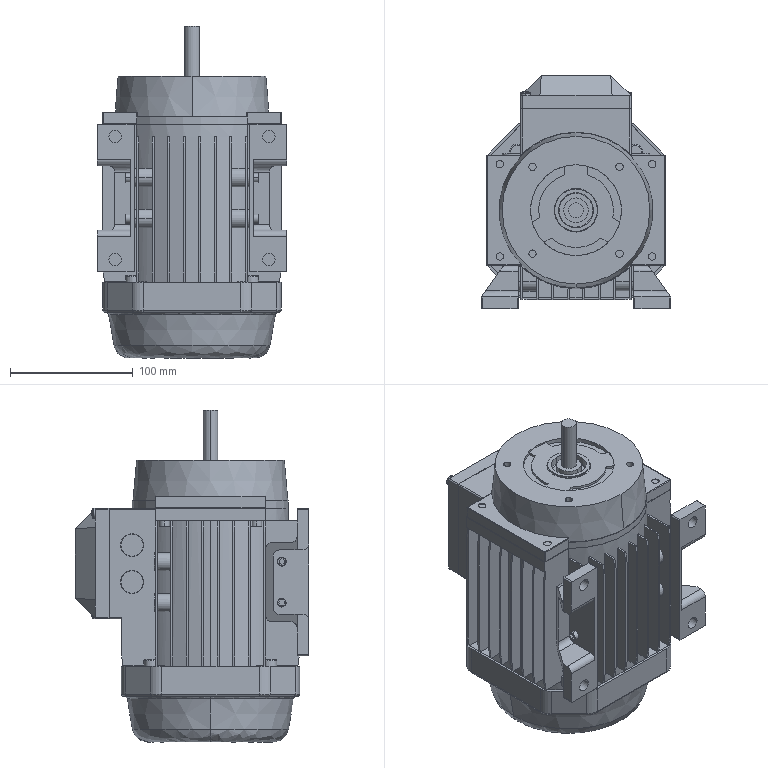Part | SolidWorks | features BaseBody 2, ICE 1 | 2 solids | 1339 faces | box 154 x 190 x 270 mm | volume 3515361 mm3 | plane 1035 | cylinder 224 | spline 68 | cone 12 | commonest cylinder face diameters 10 x34 6 x28 15 x26 2 x24 1 x16 126.999 x13